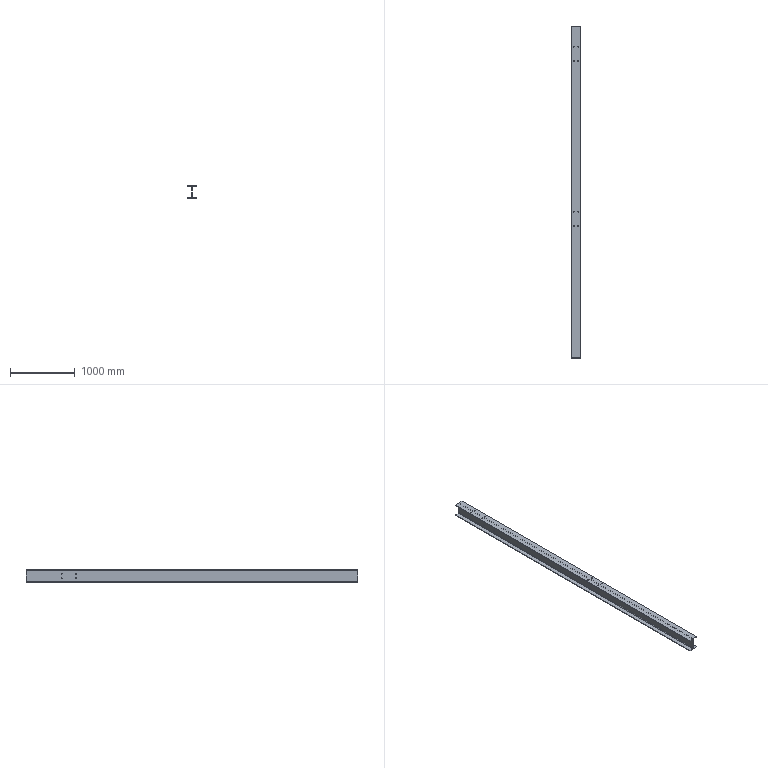Part | STEP file | 粉仓立柱1主体_Default<As Machined> | 1 solid | 42 faces | box 150 x 5128 x 194 mm | volume 19525526 mm3 | cylinder 28 | plane 14 | commonest cylinder face diameters 15 x24 16 x4